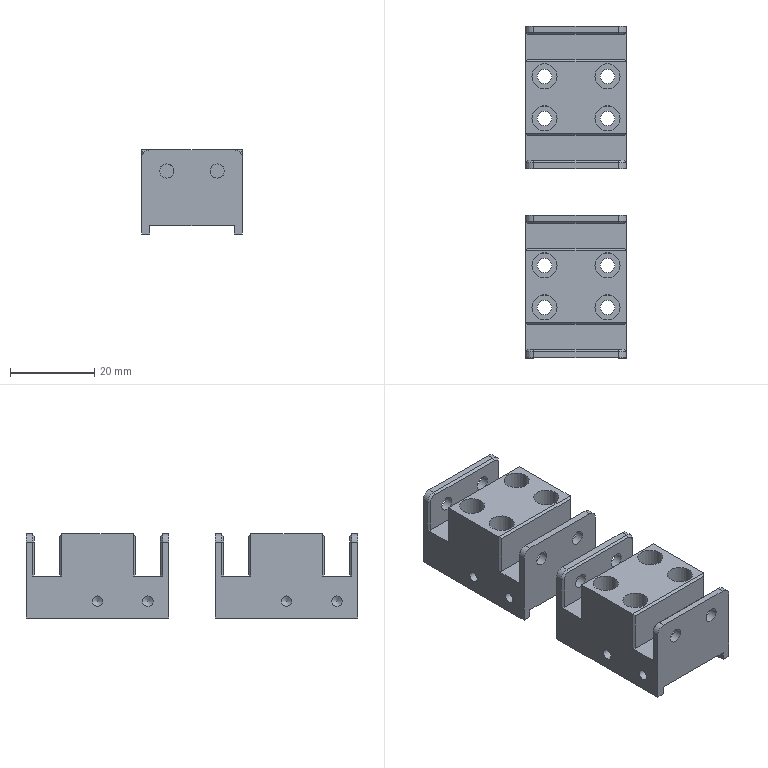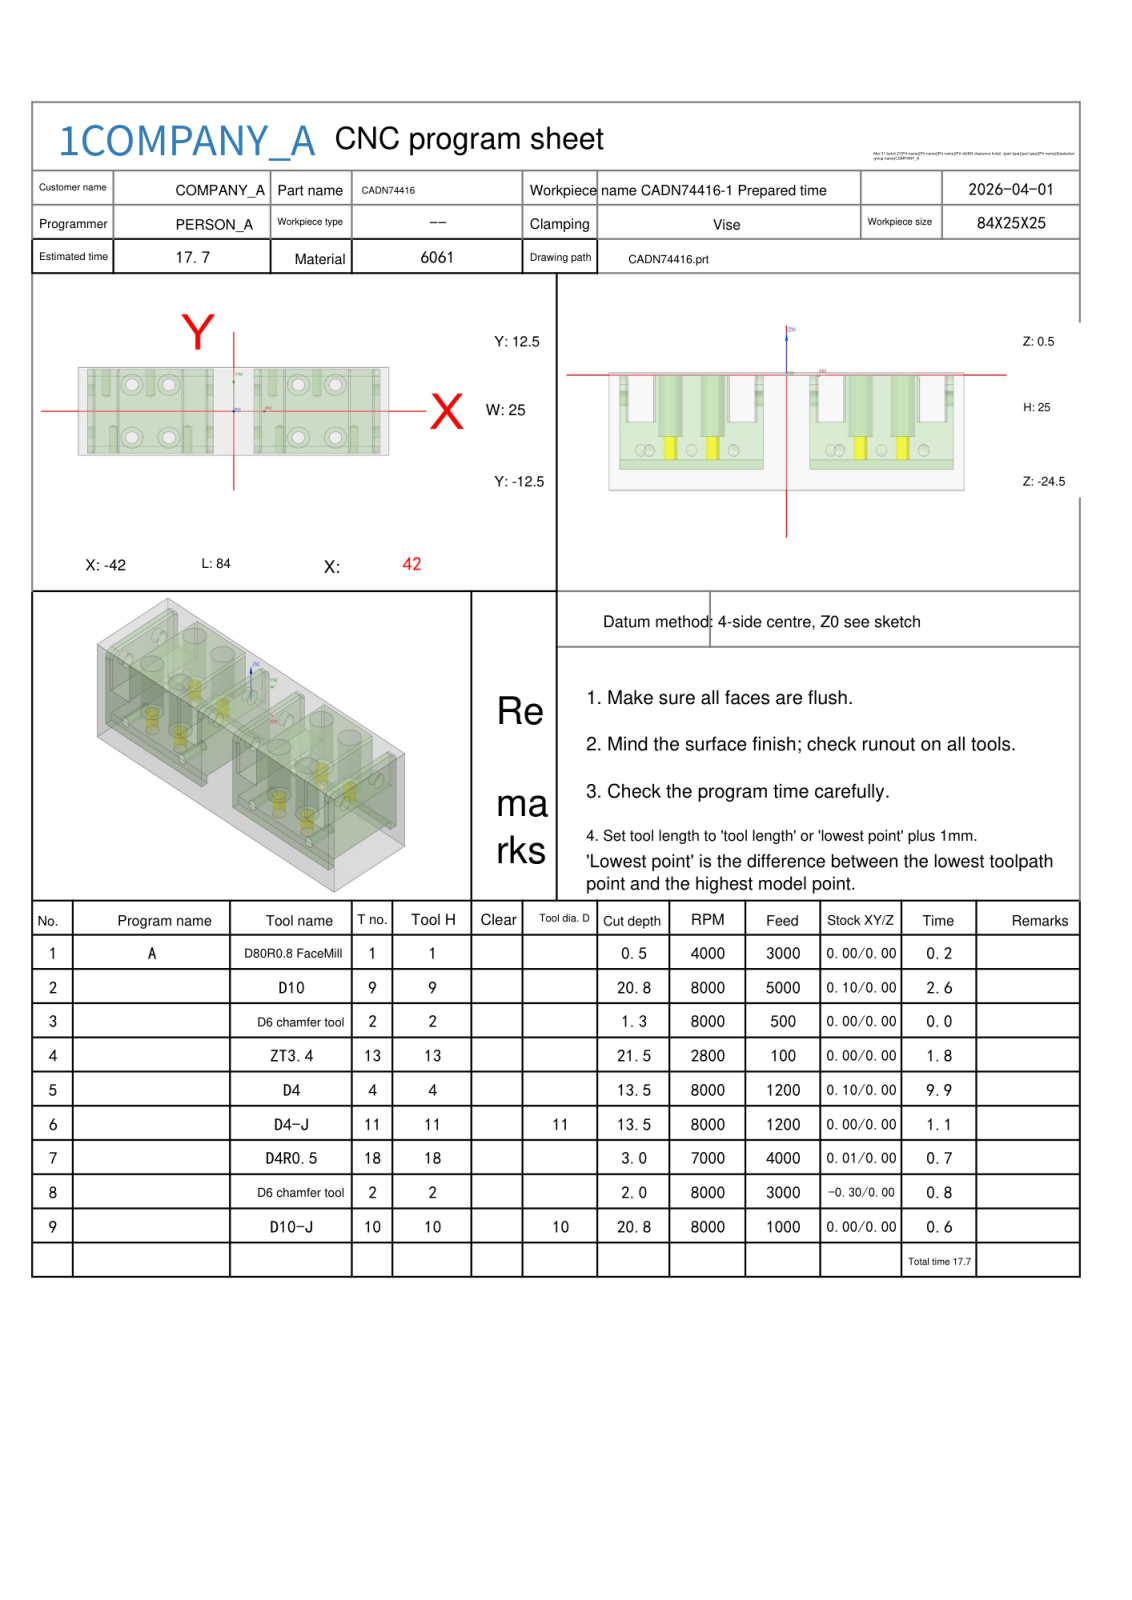NC program | NX | posted by the shop | part box 24 x 79 x 20 mm
Lines 1 to 794 of 7697:
%
O0001
(Machine time: 19.32 MIN)
(===Total Tool:8===)
(T1=D80R0.8 FaceMill D=80.  R=0.8  D-  H01 Z=-0.   )
(T9=D10     D=10.  R=0.   D-  H09 Z=-20.3 )
(T2=D6 chamfer tool   D=6.   R=0.   D-  H02 Z=-1.5  )
(T13=ZT3.4  D=3.4  DR_a=118 D-  H13 Z=-21.02)
(T4=D4      D=4.   R=0.   D-  H04 Z=-13.  )
(T11=D4-J   D=4.   R=0.   D11 H11 Z=-13.  )
(T18=D4R0.5 D=4.   R=0.5  D-  H18 Z=-2.5  )
(T10=D10-J  D=10.  R=0.   D10 H10 Z=-20.3 )
G80 G90 G17 G49 G40
G91 G28 Z0
M01
N1 T01 M06
(D80R0.8 FaceMill  D=80. R=0.8 H=01 ce=0.20 di=0.10)
G00 G90 G54 X-84.5 Y0.0 M03 S4000
G43 H01 Z20.
M08
Z2.1
G01 Z.1 F3000.
X-79.5
X79.5
X84.5
Z2.1
G00 Z20.
G00 G90 X-84.5 Y0.0 M03 S4000
Z20.
Z2.
G01 Z0.0 F1000.
X-79.5
X79.5
X84.5
Z2.
G00 Z20.
G91 G28 Z0.0
M05
M09
G91 G28 Z0.0
M01
N2 T09 M06
(D10  D=10. R=0. H=09 ce=0.10 di=0.00)
G00 G90 G54 X22.5 Y17.1 M03 S8000
G43 H09 Z20.
M08
Z.5
G01 X39.5 Z.443 F5000.
G02 X44.6 Y12. Z.416 I0.0 J-5.1
G01 Y-12. Z.336
G02 X39.5 Y-17.1 Z.309 I-5.1 J0.0
G01 X5.5 Z.196
G02 X.4 Y-12. Z.169 I0.0 J5.1
G01 Y12. Z.088
G02 X5.5 Y17.1 Z.062 I5.1 J0.0
G01 X39.5 Z-.052
G02 X44.6 Y12. Z-.079 I0.0 J-5.1
G01 Y-12. Z-.159
G02 X39.5 Y-17.1 Z-.186 I-5.1 J0.0
G01 X5.5 Z-.3
G02 X.4 Y-12. Z-.327 I0.0 J5.1
G01 Y12. Z-.407
G02 X5.5 Y17.1 Z-.434 I5.1 J0.0
G01 X39.5 Z-.547
G02 X44.6 Y12. Z-.574 I0.0 J-5.1
G01 Y-12. Z-.654
G02 X39.5 Y-17.1 Z-.681 I-5.1 J0.0
G01 X5.5 Z-.795
G02 X.4 Y-12. Z-.822 I0.0 J5.1
G01 Y12. Z-.902
G02 X5.5 Y17.1 Z-.929 I5.1 J0.0
G01 X39.5 Z-1.043
G02 X44.6 Y12. Z-1.069 I0.0 J-5.1
G01 Y-12. Z-1.15
G02 X39.5 Y-17.1 Z-1.176 I-5.1 J0.0
G01 X5.5 Z-1.29
G02 X.4 Y-12. Z-1.317 I0.0 J5.1
G01 Y12. Z-1.397
G02 X5.5 Y17.1 Z-1.424 I5.1 J0.0
G01 X39.5 Z-1.538
G02 X44.6 Y12. Z-1.565 I0.0 J-5.1
G01 Y-12. Z-1.645
G02 X39.5 Y-17.1 Z-1.672 I-5.1 J0.0
G01 X5.5 Z-1.785
G02 X.4 Y-12. Z-1.812 I0.0 J5.1
G01 Y12. Z-1.893
G02 X5.5 Y17.1 Z-1.919 I5.1 J0.0
G01 X39.5 Z-2.033
G02 X44.6 Y12. Z-2.06 I0.0 J-5.1
G01 Y-12. Z-2.14
G02 X39.5 Y-17.1 Z-2.167 I-5.1 J0.0
G01 X5.5 Z-2.281
G02 X.4 Y-12. Z-2.307 I0.0 J5.1
G01 Y12. Z-2.388
G02 X5.5 Y17.1 Z-2.415 I5.1 J0.0
G01 X39.5 Z-2.528
G02 X44.6 Y12. Z-2.555 I0.0 J-5.1
G01 Y-12. Z-2.635
G02 X39.5 Y-17.1 Z-2.662 I-5.1 J0.0
G01 X5.5 Z-2.776
G02 X.4 Y-12. Z-2.803 I0.0 J5.1
G01 Y12. Z-2.883
G02 X5.5 Y17.1 Z-2.91 I5.1 J0.0
G01 X39.5 Z-3.024
G02 X44.6 Y12. Z-3.05 I0.0 J-5.1
G01 Y-12. Z-3.131
G02 X39.5 Y-17.1 Z-3.157 I-5.1 J0.0
G01 X5.5 Z-3.271
G02 X.4 Y-12. Z-3.298 I0.0 J5.1
G01 Y12. Z-3.378
G02 X5.5 Y17.1 Z-3.405 I5.1 J0.0
G01 X39.5 Z-3.519
G02 X44.6 Y12. Z-3.546 I0.0 J-5.1
G01 Y-12. Z-3.626
G02 X39.5 Y-17.1 Z-3.653 I-5.1 J0.0
G01 X5.5 Z-3.766
G02 X.4 Y-12. Z-3.793 I0.0 J5.1
G01 Y12. Z-3.873
G02 X5.5 Y17.1 Z-3.9 I5.1 J0.0
G01 X39.5 Z-4.014
G02 X44.6 Y12. Z-4.041 I0.0 J-5.1
G01 Y-12. Z-4.121
G02 X39.5 Y-17.1 Z-4.148 I-5.1 J0.0
G01 X5.5 Z-4.262
G02 X.4 Y-12. Z-4.288 I0.0 J5.1
G01 Y12. Z-4.369
G02 X5.5 Y17.1 Z-4.396 I5.1 J0.0
G01 X39.5 Z-4.509
G02 X44.6 Y12. Z-4.536 I0.0 J-5.1
G01 Y-12. Z-4.616
G02 X39.5 Y-17.1 Z-4.643 I-5.1 J0.0
G01 X5.5 Z-4.757
G02 X.4 Y-12. Z-4.784 I0.0 J5.1
G01 Y12. Z-4.864
G02 X5.5 Y17.1 Z-4.891 I5.1 J0.0
G01 X39.5 Z-5.004
G02 X44.6 Y12. Z-5.031 I0.0 J-5.1
G01 Y-12. Z-5.112
G02 X39.5 Y-17.1 Z-5.138 I-5.1 J0.0
G01 X5.5 Z-5.252
G02 X.4 Y-12. Z-5.279 I0.0 J5.1
G01 Y12. Z-5.359
G02 X5.5 Y17.1 Z-5.386 I5.1 J0.0
G01 X39.5 Z-5.5
G02 X44.6 Y12. Z-5.527 I0.0 J-5.1
G01 Y-12. Z-5.607
G02 X39.5 Y-17.1 Z-5.634 I-5.1 J0.0
G01 X5.5 Z-5.747
G02 X.4 Y-12. Z-5.774 I0.0 J5.1
G01 Y12. Z-5.854
G02 X5.5 Y17.1 Z-5.881 I5.1 J0.0
G01 X39.5 Z-5.995
G02 X44.6 Y12. Z-6.022 I0.0 J-5.1
G01 Y-12. Z-6.102
G02 X39.5 Y-17.1 Z-6.129 I-5.1 J0.0
G01 X5.5 Z-6.243
G02 X.4 Y-12. Z-6.269 I0.0 J5.1
G01 Y12. Z-6.35
G02 X5.5 Y17.1 Z-6.376 I5.1 J0.0
G01 X39.5 Z-6.49
G02 X44.6 Y12. Z-6.517 I0.0 J-5.1
G01 Y-12. Z-6.597
G02 X39.5 Y-17.1 Z-6.624 I-5.1 J0.0
G01 X5.5 Z-6.738
G02 X.4 Y-12. Z-6.765 I0.0 J5.1
G01 Y12. Z-6.845
G02 X5.5 Y17.1 Z-6.872 I5.1 J0.0
G01 X39.5 Z-6.985
G02 X44.6 Y12. Z-7.012 I0.0 J-5.1
G01 Y-12. Z-7.093
G02 X39.5 Y-17.1 Z-7.119 I-5.1 J0.0
G01 X5.5 Z-7.233
G02 X.4 Y-12. Z-7.26 I0.0 J5.1
G01 Y12. Z-7.34
G02 X5.5 Y17.1 Z-7.367 I5.1 J0.0
G01 X39.5 Z-7.481
G02 X44.6 Y12. Z-7.507 I0.0 J-5.1
G01 Y-12. Z-7.588
G02 X39.5 Y-17.1 Z-7.615 I-5.1 J0.0
G01 X5.5 Z-7.728
G02 X.4 Y-12. Z-7.755 I0.0 J5.1
G01 Y12. Z-7.835
G02 X5.5 Y17.1 Z-7.862 I5.1 J0.0
G01 X39.5 Z-7.976
G02 X44.6 Y12. Z-8.003 I0.0 J-5.1
G01 Y-12. Z-8.083
G02 X39.5 Y-17.1 Z-8.11 I-5.1 J0.0
G01 X5.5 Z-8.224
G02 X.4 Y-12. Z-8.25 I0.0 J5.1
G01 Y12. Z-8.331
G02 X5.5 Y17.1 Z-8.357 I5.1 J0.0
G01 X39.5 Z-8.471
G02 X44.6 Y12. Z-8.498 I0.0 J-5.1
G01 Y-12. Z-8.578
G02 X39.5 Y-17.1 Z-8.605 I-5.1 J0.0
G01 X5.5 Z-8.719
G02 X.4 Y-12. Z-8.746 I0.0 J5.1
G01 Y12. Z-8.826
G02 X5.5 Y17.1 Z-8.853 I5.1 J0.0
G01 X39.5 Z-8.966
G02 X44.6 Y12. Z-8.993 I0.0 J-5.1
G01 Y-12. Z-9.073
G02 X39.5 Y-17.1 Z-9.1 I-5.1 J0.0
G01 X5.5 Z-9.214
G02 X.4 Y-12. Z-9.241 I0.0 J5.1
G01 Y12. Z-9.321
G02 X5.5 Y17.1 Z-9.348 I5.1 J0.0
G01 X39.5 Z-9.462
G02 X44.6 Y12. Z-9.488 I0.0 J-5.1
G01 Y-12. Z-9.569
G02 X39.5 Y-17.1 Z-9.596 I-5.1 J0.0
G01 X5.5 Z-9.709
G02 X.4 Y-12. Z-9.736 I0.0 J5.1
G01 Y12. Z-9.816
G02 X5.5 Y17.1 Z-9.843 I5.1 J0.0
G01 X39.5 Z-9.957
G02 X44.6 Y12. Z-9.984 I0.0 J-5.1
G01 Y-12. Z-10.064
G02 X39.5 Y-17.1 Z-10.091 I-5.1 J0.0
G01 X5.5 Z-10.204
G02 X.4 Y-12. Z-10.231 I0.0 J5.1
G01 Y12. Z-10.312
G02 X5.5 Y17.1 Z-10.338 I5.1 J0.0
G01 X39.5 Z-10.452
G02 X44.6 Y12. Z-10.479 I0.0 J-5.1
G01 Y-12. Z-10.559
G02 X39.5 Y-17.1 Z-10.586 I-5.1 J0.0
G01 X5.5 Z-10.7
G02 X.4 Y-12. Z-10.727 I0.0 J5.1
G01 Y12. Z-10.807
G02 X5.5 Y17.1 Z-10.834 I5.1 J0.0
G01 X39.5 Z-10.947
G02 X44.6 Y12. Z-10.974 I0.0 J-5.1
G01 Y-12. Z-11.054
G02 X39.5 Y-17.1 Z-11.081 I-5.1 J0.0
G01 X5.5 Z-11.195
G02 X.4 Y-12. Z-11.222 I0.0 J5.1
G01 Y12. Z-11.302
G02 X5.5 Y17.1 Z-11.329 I5.1 J0.0
G01 X39.5 Z-11.443
G02 X44.6 Y12. Z-11.469 I0.0 J-5.1
G01 Y-12. Z-11.55
G02 X39.5 Y-17.1 Z-11.576 I-5.1 J0.0
G01 X5.5 Z-11.69
G02 X.4 Y-12. Z-11.717 I0.0 J5.1
G01 Y12. Z-11.797
G02 X5.5 Y17.1 Z-11.824 I5.1 J0.0
G01 X39.5 Z-11.938
G02 X44.6 Y12. Z-11.965 I0.0 J-5.1
G01 Y-12. Z-12.045
G02 X39.5 Y-17.1 Z-12.072 I-5.1 J0.0
G01 X5.5 Z-12.185
G02 X.4 Y-12. Z-12.212 I0.0 J5.1
G01 Y12. Z-12.293
G02 X5.5 Y17.1 Z-12.319 I5.1 J0.0
G01 X39.5 Z-12.433
G02 X44.6 Y12. Z-12.46 I0.0 J-5.1
G01 Y-12. Z-12.54
G02 X39.5 Y-17.1 Z-12.567 I-5.1 J0.0
G01 X5.5 Z-12.681
G02 X.4 Y-12. Z-12.707 I0.0 J5.1
G01 Y12. Z-12.788
G02 X5.5 Y17.1 Z-12.815 I5.1 J0.0
G01 X39.5 Z-12.928
G02 X44.6 Y12. Z-12.955 I0.0 J-5.1
G01 Y-12. Z-13.035
G02 X39.5 Y-17.1 Z-13.062 I-5.1 J0.0
G01 X5.5 Z-13.176
G02 X.4 Y-12. Z-13.203 I0.0 J5.1
G01 Y12. Z-13.283
G02 X5.5 Y17.1 Z-13.31 I5.1 J0.0
G01 X39.5 Z-13.424
G02 X44.6 Y12. Z-13.45 I0.0 J-5.1
G01 Y-12. Z-13.531
G02 X39.5 Y-17.1 Z-13.557 I-5.1 J0.0
G01 X5.5 Z-13.671
G02 X.4 Y-12. Z-13.698 I0.0 J5.1
G01 Y12. Z-13.778
G02 X5.5 Y17.1 Z-13.805 I5.1 J0.0
G01 X39.5 Z-13.919
G02 X44.6 Y12. Z-13.946 I0.0 J-5.1
G01 Y-12. Z-14.026
G02 X39.5 Y-17.1 Z-14.053 I-5.1 J0.0
G01 X5.5 Z-14.166
G02 X.4 Y-12. Z-14.193 I0.0 J5.1
G01 Y12. Z-14.273
G02 X5.5 Y17.1 Z-14.3 I5.1 J0.0
G01 X39.5 Z-14.414
G02 X44.6 Y12. Z-14.441 I0.0 J-5.1
G01 Y-12. Z-14.521
G02 X39.5 Y-17.1 Z-14.548 I-5.1 J0.0
G01 X5.5 Z-14.662
G02 X.4 Y-12. Z-14.688 I0.0 J5.1
G01 Y12. Z-14.769
G02 X5.5 Y17.1 Z-14.796 I5.1 J0.0
G01 X39.5 Z-14.909
G02 X44.6 Y12. Z-14.936 I0.0 J-5.1
G01 Y-12. Z-15.016
G02 X39.5 Y-17.1 Z-15.043 I-5.1 J0.0
G01 X5.5 Z-15.157
G02 X.4 Y-12. Z-15.184 I0.0 J5.1
G01 Y12. Z-15.264
G02 X5.5 Y17.1 Z-15.291 I5.1 J0.0
G01 X39.5 Z-15.404
G02 X44.6 Y12. Z-15.431 I0.0 J-5.1
G01 Y-12. Z-15.512
G02 X39.5 Y-17.1 Z-15.538 I-5.1 J0.0
G01 X5.5 Z-15.652
G02 X.4 Y-12. Z-15.679 I0.0 J5.1
G01 Y12. Z-15.759
G02 X5.5 Y17.1 Z-15.786 I5.1 J0.0
G01 X39.5 Z-15.9
G02 X44.6 Y12. Z-15.927 I0.0 J-5.1
G01 Y-12. Z-16.007
G02 X39.5 Y-17.1 Z-16.034 I-5.1 J0.0
G01 X5.5 Z-16.147
G02 X.4 Y-12. Z-16.174 I0.0 J5.1
G01 Y12. Z-16.254
G02 X5.5 Y17.1 Z-16.281 I5.1 J0.0
G01 X39.5 Z-16.395
G02 X44.6 Y12. Z-16.422 I0.0 J-5.1
G01 Y-12. Z-16.502
G02 X39.5 Y-17.1 Z-16.529 I-5.1 J0.0
G01 X5.5 Z-16.643
G02 X.4 Y-12. Z-16.669 I0.0 J5.1
G01 Y12. Z-16.75
G02 X5.5 Y17.1 Z-16.776 I5.1 J0.0
G01 X39.5 Z-16.89
G02 X44.6 Y12. Z-16.917 I0.0 J-5.1
G01 Y-12. Z-16.997
G02 X39.5 Y-17.1 Z-17.024 I-5.1 J0.0
G01 X5.5 Z-17.138
G02 X.4 Y-12. Z-17.165 I0.0 J5.1
G01 Y12. Z-17.245
G02 X5.5 Y17.1 Z-17.272 I5.1 J0.0
G01 X39.5 Z-17.385
G02 X44.6 Y12. Z-17.412 I0.0 J-5.1
G01 Y-12. Z-17.493
G02 X39.5 Y-17.1 Z-17.519 I-5.1 J0.0
G01 X5.5 Z-17.633
G02 X.4 Y-12. Z-17.66 I0.0 J5.1
G01 Y12. Z-17.74
G02 X5.5 Y17.1 Z-17.767 I5.1 J0.0
G01 X39.5 Z-17.881
G02 X44.6 Y12. Z-17.907 I0.0 J-5.1
G01 Y-12. Z-17.988
G02 X39.5 Y-17.1 Z-18.015 I-5.1 J0.0
G01 X5.5 Z-18.128
G02 X.4 Y-12. Z-18.155 I0.0 J5.1
G01 Y12. Z-18.235
G02 X5.5 Y17.1 Z-18.262 I5.1 J0.0
G01 X39.5 Z-18.376
G02 X44.6 Y12. Z-18.403 I0.0 J-5.1
G01 Y-12. Z-18.483
G02 X39.5 Y-17.1 Z-18.51 I-5.1 J0.0
G01 X5.5 Z-18.624
G02 X.4 Y-12. Z-18.65 I0.0 J5.1
G01 Y12. Z-18.731
G02 X5.5 Y17.1 Z-18.757 I5.1 J0.0
G01 X39.5 Z-18.871
G02 X44.6 Y12. Z-18.898 I0.0 J-5.1
G01 Y-12. Z-18.978
G02 X39.5 Y-17.1 Z-19.005 I-5.1 J0.0
G01 X5.5 Z-19.119
G02 X.4 Y-12. Z-19.146 I0.0 J5.1
G01 Y12. Z-19.226
G02 X5.5 Y17.1 Z-19.253 I5.1 J0.0
G01 X39.5 Z-19.366
G02 X44.6 Y12. Z-19.393 I0.0 J-5.1
G01 Y-12. Z-19.473
G02 X39.5 Y-17.1 Z-19.5 I-5.1 J0.0
G01 X5.5 Z-19.614
G02 X.4 Y-12. Z-19.641 I0.0 J5.1
G01 Y12. Z-19.721
G02 X5.5 Y17.1 Z-19.748 I5.1 J0.0
G01 X39.5 Z-19.862
G02 X44.6 Y12. Z-19.888 I0.0 J-5.1
G01 Y-12. Z-19.969
G02 X39.5 Y-17.1 Z-19.996 I-5.1 J0.0
G01 X5.5 Z-20.109
G02 X.4 Y-12. Z-20.136 I0.0 J5.1
G01 Y12. Z-20.216
G02 X5.5 Y17.1 Z-20.243 I5.1 J0.0
G01 X22.5 Z-20.3
X39.5
G02 X44.6 Y12. I0.0 J-5.1
G01 Y-12.
G02 X39.5 Y-17.1 I-5.1 J0.0
G01 X5.5
G02 X.4 Y-12. I0.0 J5.1
G01 Y12.
G02 X5.5 Y17.1 I5.1 J0.0
G01 X22.5
X23.
Z-19.3
G00 Z20.
X-22.5
Z.5
G01 X-5.5 Z.443
G02 X-.4 Y12. Z.416 I0.0 J-5.1
G01 Y-12. Z.336
G02 X-5.5 Y-17.1 Z.309 I-5.1 J0.0
G01 X-39.5 Z.196
G02 X-44.6 Y-12. Z.169 I0.0 J5.1
G01 Y12. Z.088
G02 X-39.5 Y17.1 Z.062 I5.1 J0.0
G01 X-5.5 Z-.052
G02 X-.4 Y12. Z-.079 I0.0 J-5.1
G01 Y-12. Z-.159
G02 X-5.5 Y-17.1 Z-.186 I-5.1 J0.0
G01 X-39.5 Z-.3
G02 X-44.6 Y-12. Z-.327 I0.0 J5.1
G01 Y12. Z-.407
G02 X-39.5 Y17.1 Z-.434 I5.1 J0.0
G01 X-5.5 Z-.547
G02 X-.4 Y12. Z-.574 I0.0 J-5.1
G01 Y-12. Z-.654
G02 X-5.5 Y-17.1 Z-.681 I-5.1 J0.0
G01 X-39.5 Z-.795
G02 X-44.6 Y-12. Z-.822 I0.0 J5.1
G01 Y12. Z-.902
G02 X-39.5 Y17.1 Z-.929 I5.1 J0.0
G01 X-5.5 Z-1.043
G02 X-.4 Y12. Z-1.069 I0.0 J-5.1
G01 Y-12. Z-1.15
G02 X-5.5 Y-17.1 Z-1.176 I-5.1 J0.0
G01 X-39.5 Z-1.29
G02 X-44.6 Y-12. Z-1.317 I0.0 J5.1
G01 Y12. Z-1.397
G02 X-39.5 Y17.1 Z-1.424 I5.1 J0.0
G01 X-5.5 Z-1.538
G02 X-.4 Y12. Z-1.565 I0.0 J-5.1
G01 Y-12. Z-1.645
G02 X-5.5 Y-17.1 Z-1.672 I-5.1 J0.0
G01 X-39.5 Z-1.785
G02 X-44.6 Y-12. Z-1.812 I0.0 J5.1
G01 Y12. Z-1.893
G02 X-39.5 Y17.1 Z-1.919 I5.1 J0.0
G01 X-5.5 Z-2.033
G02 X-.4 Y12. Z-2.06 I0.0 J-5.1
G01 Y-12. Z-2.14
G02 X-5.5 Y-17.1 Z-2.167 I-5.1 J0.0
G01 X-39.5 Z-2.281
G02 X-44.6 Y-12. Z-2.307 I0.0 J5.1
G01 Y12. Z-2.388
G02 X-39.5 Y17.1 Z-2.415 I5.1 J0.0
G01 X-5.5 Z-2.528
G02 X-.4 Y12. Z-2.555 I0.0 J-5.1
G01 Y-12. Z-2.635
G02 X-5.5 Y-17.1 Z-2.662 I-5.1 J0.0
G01 X-39.5 Z-2.776
G02 X-44.6 Y-12. Z-2.803 I0.0 J5.1
G01 Y12. Z-2.883
G02 X-39.5 Y17.1 Z-2.91 I5.1 J0.0
G01 X-5.5 Z-3.024
G02 X-.4 Y12. Z-3.05 I0.0 J-5.1
G01 Y-12. Z-3.131
G02 X-5.5 Y-17.1 Z-3.157 I-5.1 J0.0
G01 X-39.5 Z-3.271
G02 X-44.6 Y-12. Z-3.298 I0.0 J5.1
G01 Y12. Z-3.378
G02 X-39.5 Y17.1 Z-3.405 I5.1 J0.0
G01 X-5.5 Z-3.519
G02 X-.4 Y12. Z-3.546 I0.0 J-5.1
G01 Y-12. Z-3.626
G02 X-5.5 Y-17.1 Z-3.653 I-5.1 J0.0
G01 X-39.5 Z-3.766
G02 X-44.6 Y-12. Z-3.793 I0.0 J5.1
G01 Y12. Z-3.873
G02 X-39.5 Y17.1 Z-3.9 I5.1 J0.0
G01 X-5.5 Z-4.014
G02 X-.4 Y12. Z-4.041 I0.0 J-5.1
G01 Y-12. Z-4.121
G02 X-5.5 Y-17.1 Z-4.148 I-5.1 J0.0
G01 X-39.5 Z-4.262
G02 X-44.6 Y-12. Z-4.288 I0.0 J5.1
G01 Y12. Z-4.369
G02 X-39.5 Y17.1 Z-4.396 I5.1 J0.0
G01 X-5.5 Z-4.509
G02 X-.4 Y12. Z-4.536 I0.0 J-5.1
G01 Y-12. Z-4.616
G02 X-5.5 Y-17.1 Z-4.643 I-5.1 J0.0
G01 X-39.5 Z-4.757
G02 X-44.6 Y-12. Z-4.784 I0.0 J5.1
G01 Y12. Z-4.864
G02 X-39.5 Y17.1 Z-4.891 I5.1 J0.0
G01 X-5.5 Z-5.004
G02 X-.4 Y12. Z-5.031 I0.0 J-5.1
G01 Y-12. Z-5.112
G02 X-5.5 Y-17.1 Z-5.138 I-5.1 J0.0
G01 X-39.5 Z-5.252
G02 X-44.6 Y-12. Z-5.279 I0.0 J5.1
G01 Y12. Z-5.359
G02 X-39.5 Y17.1 Z-5.386 I5.1 J0.0
G01 X-5.5 Z-5.5
G02 X-.4 Y12. Z-5.527 I0.0 J-5.1
G01 Y-12. Z-5.607
G02 X-5.5 Y-17.1 Z-5.634 I-5.1 J0.0
G01 X-39.5 Z-5.747
G02 X-44.6 Y-12. Z-5.774 I0.0 J5.1
G01 Y12. Z-5.854
G02 X-39.5 Y17.1 Z-5.881 I5.1 J0.0
G01 X-5.5 Z-5.995
G02 X-.4 Y12. Z-6.022 I0.0 J-5.1
G01 Y-12. Z-6.102
G02 X-5.5 Y-17.1 Z-6.129 I-5.1 J0.0
G01 X-39.5 Z-6.243
G02 X-44.6 Y-12. Z-6.269 I0.0 J5.1
G01 Y12. Z-6.35
G02 X-39.5 Y17.1 Z-6.376 I5.1 J0.0
G01 X-5.5 Z-6.49
G02 X-.4 Y12. Z-6.517 I0.0 J-5.1
G01 Y-12. Z-6.597
G02 X-5.5 Y-17.1 Z-6.624 I-5.1 J0.0
G01 X-39.5 Z-6.738
G02 X-44.6 Y-12. Z-6.765 I0.0 J5.1
G01 Y12. Z-6.845
G02 X-39.5 Y17.1 Z-6.872 I5.1 J0.0
G01 X-5.5 Z-6.985
G02 X-.4 Y12. Z-7.012 I0.0 J-5.1
G01 Y-12. Z-7.093
G02 X-5.5 Y-17.1 Z-7.119 I-5.1 J0.0
G01 X-39.5 Z-7.233
G02 X-44.6 Y-12. Z-7.26 I0.0 J5.1
G01 Y12. Z-7.34
G02 X-39.5 Y17.1 Z-7.367 I5.1 J0.0
G01 X-5.5 Z-7.481
G02 X-.4 Y12. Z-7.507 I0.0 J-5.1
G01 Y-12. Z-7.588
G02 X-5.5 Y-17.1 Z-7.615 I-5.1 J0.0
G01 X-39.5 Z-7.728
G02 X-44.6 Y-12. Z-7.755 I0.0 J5.1
G01 Y12. Z-7.835
G02 X-39.5 Y17.1 Z-7.862 I5.1 J0.0
G01 X-5.5 Z-7.976
G02 X-.4 Y12. Z-8.003 I0.0 J-5.1
G01 Y-12. Z-8.083
G02 X-5.5 Y-17.1 Z-8.11 I-5.1 J0.0
G01 X-39.5 Z-8.224
G02 X-44.6 Y-12. Z-8.25 I0.0 J5.1
G01 Y12. Z-8.331
G02 X-39.5 Y17.1 Z-8.357 I5.1 J0.0
G01 X-5.5 Z-8.471
G02 X-.4 Y12. Z-8.498 I0.0 J-5.1
G01 Y-12. Z-8.578
G02 X-5.5 Y-17.1 Z-8.605 I-5.1 J0.0
G01 X-39.5 Z-8.719
G02 X-44.6 Y-12. Z-8.746 I0.0 J5.1
G01 Y12. Z-8.826
G02 X-39.5 Y17.1 Z-8.853 I5.1 J0.0
G01 X-5.5 Z-8.966
G02 X-.4 Y12. Z-8.993 I0.0 J-5.1
G01 Y-12. Z-9.073
G02 X-5.5 Y-17.1 Z-9.1 I-5.1 J0.0
G01 X-39.5 Z-9.214
G02 X-44.6 Y-12. Z-9.241 I0.0 J5.1
G01 Y12. Z-9.321
G02 X-39.5 Y17.1 Z-9.348 I5.1 J0.0
G01 X-5.5 Z-9.462
G02 X-.4 Y12. Z-9.488 I0.0 J-5.1
G01 Y-12. Z-9.569
G02 X-5.5 Y-17.1 Z-9.596 I-5.1 J0.0
G01 X-39.5 Z-9.709
G02 X-44.6 Y-12. Z-9.736 I0.0 J5.1
G01 Y12. Z-9.816
G02 X-39.5 Y17.1 Z-9.843 I5.1 J0.0
G01 X-5.5 Z-9.957
G02 X-.4 Y12. Z-9.984 I0.0 J-5.1
G01 Y-12. Z-10.064
G02 X-5.5 Y-17.1 Z-10.091 I-5.1 J0.0
G01 X-39.5 Z-10.204
G02 X-44.6 Y-12. Z-10.231 I0.0 J5.1
G01 Y12. Z-10.312
G02 X-39.5 Y17.1 Z-10.338 I5.1 J0.0
G01 X-5.5 Z-10.452
G02 X-.4 Y12. Z-10.479 I0.0 J-5.1
G01 Y-12. Z-10.559
G02 X-5.5 Y-17.1 Z-10.586 I-5.1 J0.0
G01 X-39.5 Z-10.7
G02 X-44.6 Y-12. Z-10.727 I0.0 J5.1
G01 Y12. Z-10.807
G02 X-39.5 Y17.1 Z-10.834 I5.1 J0.0
G01 X-5.5 Z-10.947
G02 X-.4 Y12. Z-10.974 I0.0 J-5.1
G01 Y-12. Z-11.054
G02 X-5.5 Y-17.1 Z-11.081 I-5.1 J0.0
G01 X-39.5 Z-11.195
G02 X-44.6 Y-12. Z-11.222 I0.0 J5.1
G01 Y12. Z-11.302
G02 X-39.5 Y17.1 Z-11.329 I5.1 J0.0
G01 X-5.5 Z-11.443
G02 X-.4 Y12. Z-11.469 I0.0 J-5.1
G01 Y-12. Z-11.55
G02 X-5.5 Y-17.1 Z-11.576 I-5.1 J0.0
G01 X-39.5 Z-11.69
G02 X-44.6 Y-12. Z-11.717 I0.0 J5.1
G01 Y12. Z-11.797
G02 X-39.5 Y17.1 Z-11.824 I5.1 J0.0
G01 X-5.5 Z-11.938
G02 X-.4 Y12. Z-11.965 I0.0 J-5.1
G01 Y-12. Z-12.045
G02 X-5.5 Y-17.1 Z-12.072 I-5.1 J0.0
G01 X-39.5 Z-12.185
G02 X-44.6 Y-12. Z-12.212 I0.0 J5.1
G01 Y12. Z-12.293
G02 X-39.5 Y17.1 Z-12.319 I5.1 J0.0
G01 X-5.5 Z-12.433
G02 X-.4 Y12. Z-12.46 I0.0 J-5.1
G01 Y-12. Z-12.54
G02 X-5.5 Y-17.1 Z-12.567 I-5.1 J0.0
G01 X-39.5 Z-12.681
G02 X-44.6 Y-12. Z-12.707 I0.0 J5.1
G01 Y12. Z-12.788
G02 X-39.5 Y17.1 Z-12.815 I5.1 J0.0
G01 X-5.5 Z-12.928
G02 X-.4 Y12. Z-12.955 I0.0 J-5.1
G01 Y-12. Z-13.035
G02 X-5.5 Y-17.1 Z-13.062 I-5.1 J0.0
G01 X-39.5 Z-13.176
G02 X-44.6 Y-12. Z-13.203 I0.0 J5.1
G01 Y12. Z-13.283
G02 X-39.5 Y17.1 Z-13.31 I5.1 J0.0
G01 X-5.5 Z-13.424
G02 X-.4 Y12. Z-13.45 I0.0 J-5.1
G01 Y-12. Z-13.531
G02 X-5.5 Y-17.1 Z-13.557 I-5.1 J0.0
G01 X-39.5 Z-13.671
G02 X-44.6 Y-12. Z-13.698 I0.0 J5.1
G01 Y12. Z-13.778
G02 X-39.5 Y17.1 Z-13.805 I5.1 J0.0
G01 X-5.5 Z-13.919
G02 X-.4 Y12. Z-13.946 I0.0 J-5.1
G01 Y-12. Z-14.026
G02 X-5.5 Y-17.1 Z-14.053 I-5.1 J0.0
G01 X-39.5 Z-14.166
G02 X-44.6 Y-12. Z-14.193 I0.0 J5.1
G01 Y12. Z-14.273
G02 X-39.5 Y17.1 Z-14.3 I5.1 J0.0
G01 X-5.5 Z-14.414
G02 X-.4 Y12. Z-14.441 I0.0 J-5.1
G01 Y-12. Z-14.521
G02 X-5.5 Y-17.1 Z-14.548 I-5.1 J0.0
G01 X-39.5 Z-14.662
G02 X-44.6 Y-12. Z-14.688 I0.0 J5.1
G01 Y12. Z-14.769
G02 X-39.5 Y17.1 Z-14.796 I5.1 J0.0
G01 X-5.5 Z-14.909
G02 X-.4 Y12. Z-14.936 I0.0 J-5.1
G01 Y-12. Z-15.016
G02 X-5.5 Y-17.1 Z-15.043 I-5.1 J0.0
G01 X-39.5 Z-15.157
G02 X-44.6 Y-12. Z-15.184 I0.0 J5.1
G01 Y12. Z-15.264
G02 X-39.5 Y17.1 Z-15.291 I5.1 J0.0
G01 X-5.5 Z-15.404
G02 X-.4 Y12. Z-15.431 I0.0 J-5.1
G01 Y-12. Z-15.512
G02 X-5.5 Y-17.1 Z-15.538 I-5.1 J0.0
G01 X-39.5 Z-15.652
G02 X-44.6 Y-12. Z-15.679 I0.0 J5.1
G01 Y12. Z-15.759
G02 X-39.5 Y17.1 Z-15.786 I5.1 J0.0
G01 X-5.5 Z-15.9
G02 X-.4 Y12. Z-15.927 I0.0 J-5.1
G01 Y-12. Z-16.007
G02 X-5.5 Y-17.1 Z-16.034 I-5.1 J0.0
G01 X-39.5 Z-16.147
G02 X-44.6 Y-12. Z-16.174 I0.0 J5.1
G01 Y12. Z-16.254
G02 X-39.5 Y17.1 Z-16.281 I5.1 J0.0
G01 X-5.5 Z-16.395
G02 X-.4 Y12. Z-16.422 I0.0 J-5.1
G01 Y-12. Z-16.502
G02 X-5.5 Y-17.1 Z-16.529 I-5.1 J0.0
G01 X-39.5 Z-16.643
G02 X-44.6 Y-12. Z-16.669 I0.0 J5.1
G01 Y12. Z-16.75
G02 X-39.5 Y17.1 Z-16.776 I5.1 J0.0
G01 X-5.5 Z-16.89
G02 X-.4 Y12. Z-16.917 I0.0 J-5.1
G01 Y-12. Z-16.997
G02 X-5.5 Y-17.1 Z-17.024 I-5.1 J0.0
G01 X-39.5 Z-17.138
G02 X-44.6 Y-12. Z-17.165 I0.0 J5.1
G01 Y12. Z-17.245
G02 X-39.5 Y17.1 Z-17.272 I5.1 J0.0
G01 X-5.5 Z-17.385
G02 X-.4 Y12. Z-17.412 I0.0 J-5.1
G01 Y-12. Z-17.493
G02 X-5.5 Y-17.1 Z-17.519 I-5.1 J0.0
G01 X-39.5 Z-17.633
G02 X-44.6 Y-12. Z-17.66 I0.0 J5.1
G01 Y12. Z-17.74
G02 X-39.5 Y17.1 Z-17.767 I5.1 J0.0
G01 X-5.5 Z-17.881
G02 X-.4 Y12. Z-17.907 I0.0 J-5.1
G01 Y-12. Z-17.988
G02 X-5.5 Y-17.1 Z-18.015 I-5.1 J0.0
G01 X-39.5 Z-18.128
G02 X-44.6 Y-12. Z-18.155 I0.0 J5.1
G01 Y12. Z-18.235
G02 X-39.5 Y17.1 Z-18.262 I5.1 J0.0
G01 X-5.5 Z-18.376
G02 X-.4 Y12. Z-18.403 I0.0 J-5.1
G01 Y-12. Z-18.483
G02 X-5.5 Y-17.1 Z-18.51 I-5.1 J0.0
G01 X-39.5 Z-18.624
G02 X-44.6 Y-12. Z-18.65 I0.0 J5.1
G01 Y12. Z-18.731
G02 X-39.5 Y17.1 Z-18.757 I5.1 J0.0
G01 X-5.5 Z-18.871
G02 X-.4 Y12. Z-18.898 I0.0 J-5.1
G01 Y-12. Z-18.978
G02 X-5.5 Y-17.1 Z-19.005 I-5.1 J0.0
G01 X-39.5 Z-19.119
G02 X-44.6 Y-12. Z-19.146 I0.0 J5.1
G01 Y12. Z-19.226
G02 X-39.5 Y17.1 Z-19.253 I5.1 J0.0
G01 X-5.5 Z-19.366
G02 X-.4 Y12. Z-19.393 I0.0 J-5.1
G01 Y-12. Z-19.473
G02 X-5.5 Y-17.1 Z-19.5 I-5.1 J0.0
G01 X-39.5 Z-19.614
G02 X-44.6 Y-12. Z-19.641 I0.0 J5.1
G01 Y12. Z-19.721
G02 X-39.5 Y17.1 Z-19.748 I5.1 J0.0
G01 X-5.5 Z-19.862
G02 X-.4 Y12. Z-19.888 I0.0 J-5.1
G01 Y-12. Z-19.969
G02 X-5.5 Y-17.1 Z-19.996 I-5.1 J0.0
G01 X-39.5 Z-20.109
G02 X-44.6 Y-12. Z-20.136 I0.0 J5.1
G01 Y12. Z-20.216
G02 X-39.5 Y17.1 Z-20.243 I5.1 J0.0
G01 X-22.5 Z-20.3
X-5.5
G02 X-.4 Y12. I0.0 J-5.1
G01 Y-12.
G02 X-5.5 Y-17.1 I-5.1 J0.0
G01 X-39.5
G02 X-44.6 Y-12. I0.0 J5.1
G01 Y12.
G02 X-39.5 Y17.1 I5.1 J0.0
G01 X-22.5
X-22.
Z-19.3
G00 Z20.
G91 G28 Z0.0
M05
M09
G91 G28 Z0.0
M01
N3 T02 M06
(D6 chamfer tool  D=6. R=0. H=02 ce=0.00 di=0.00)
G00 G90 G54 X17.5 Y-7.5 M03 S8000
G43 H02 Z20.
M08
G98 G81 X17.5 Y-7.5 Z-.8 R1. F500.
X27.5
Y7.5
X17.5
X-17.5
X-27.5
Y-7.5
X-17.5
G80
G00 Z20.
G91 G28 Z0.0
M05
M09
G91 G28 Z0.0
M01
N4 T13 M06
(ZT3.4 D=3.4 DR_a=118 H=13)
G00 G90 G54 X17.5 Y-7.5 M03 S2800
G43 H13 Z20.
M08
G98 G83 X17.5 Y-7.5 Z-21.021 R1. F100. Q2.
X27.5
Y7.5
X17.5
X-17.5
X-27.5
Y-7.5
X-17.5
G80
G00 Z20.
G91 G28 Z0.0
M05
M09
G91 G28 Z0.0
M01